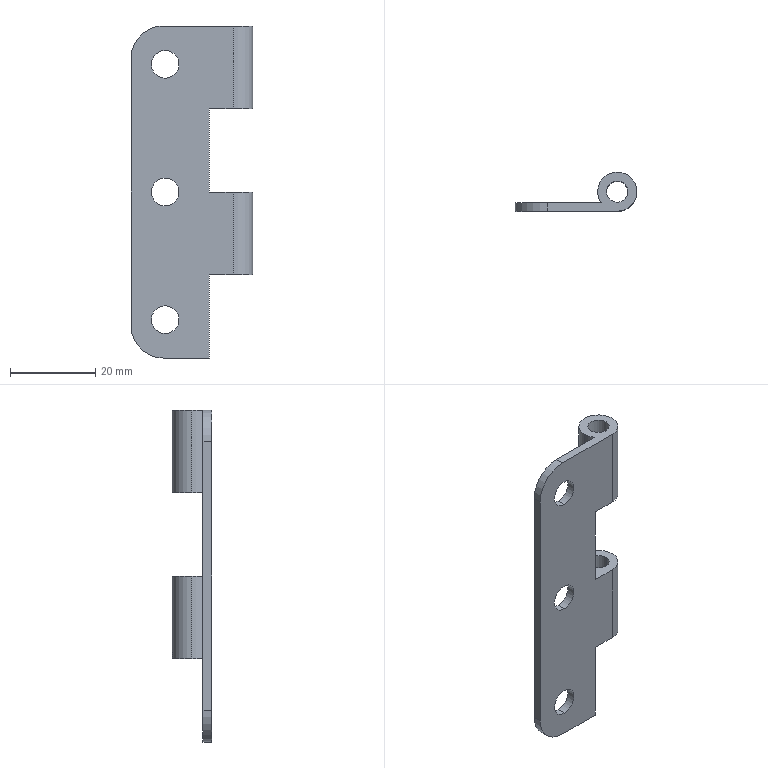Part | SolidWorks | features BaseBody 1 | 1 solid | 28 faces | box 28.6 x 9.2 x 78 mm | volume 4679 mm3 | cylinder 18 | plane 10 | commonest cylinder face diameters 6.5 x6 9.2 x6 5 x4 15 x2
STEP:
#1=CARTESIAN_POINT('',(-16.,2.,-33.25));
#2=VERTEX_POINT('',#1);
#3=CARTESIAN_POINT('',(-16.,2.,-26.75));
#4=VERTEX_POINT('',#3);
#5=CARTESIAN_POINT('',(-16.,2.,-30.));
#6=DIRECTION('',(0.,1.,0.));
#7=DIRECTION('',(0.,0.,1.));
#8=AXIS2_PLACEMENT_3D('',#5,#6,#7);
#9=CIRCLE('',#8,3.25);
#10=EDGE_CURVE('',#2,#4,#9,.T.);
#11=ORIENTED_EDGE('',*,*,#10,.T.);
#12=CARTESIAN_POINT('',(-16.,0.,-26.75));
#13=VERTEX_POINT('',#12);
#14=CARTESIAN_POINT('',(-16.,2.,-26.75));
#15=DIRECTION('',(0.,-1.,0.));
#16=VECTOR('',#15,1000.);
#17=LINE('',#14,#16);
#18=EDGE_CURVE('',#4,#13,#17,.T.);
#19=ORIENTED_EDGE('',*,*,#18,.T.);
#20=CARTESIAN_POINT('',(-16.,0.,-33.25));
#21=VERTEX_POINT('',#20);
#22=CARTESIAN_POINT('',(-16.,0.,-30.));
#23=DIRECTION('',(0.,1.,0.));
#24=DIRECTION('',(0.,0.,1.));
#25=AXIS2_PLACEMENT_3D('',#22,#23,#24);
#26=CIRCLE('',#25,3.25);
#27=EDGE_CURVE('',#21,#13,#26,.T.);
#28=ORIENTED_EDGE('',*,*,#27,.F.);
#29=CARTESIAN_POINT('',(-16.,2.,-33.25));
#30=DIRECTION('',(0.,-1.,0.));
#31=VECTOR('',#30,1000.);
#32=LINE('',#29,#31);
#33=EDGE_CURVE('',#2,#21,#32,.T.);
#34=ORIENTED_EDGE('',*,*,#33,.F.);
#35=EDGE_LOOP('',(#11,#19,#28,#34));
#36=FACE_OUTER_BOUND('',#35,.T.);
#37=CARTESIAN_POINT('',(-16.,2.,-30.));
#38=DIRECTION('',(0.,-1.,0.));
#39=DIRECTION('',(0.,0.,-1.));
#40=AXIS2_PLACEMENT_3D('',#37,#38,#39);
#41=CYLINDRICAL_SURFACE('',#40,3.25);
#42=ADVANCED_FACE('',(#36),#41,.F.);
#43=CARTESIAN_POINT('',(-16.,2.,26.75));
#44=VERTEX_POINT('',#43);
#45=CARTESIAN_POINT('',(-16.,2.,33.25));
#46=VERTEX_POINT('',#45);
#47=CARTESIAN_POINT('',(-16.,2.,30.));
#48=DIRECTION('',(0.,1.,0.));
#49=DIRECTION('',(0.,0.,1.));
#50=AXIS2_PLACEMENT_3D('',#47,#48,#49);
#51=CIRCLE('',#50,3.25);
#52=EDGE_CURVE('',#44,#46,#51,.T.);
#53=ORIENTED_EDGE('',*,*,#52,.T.);
#54=CARTESIAN_POINT('',(-16.,0.,33.25));
#55=VERTEX_POINT('',#54);
#56=CARTESIAN_POINT('',(-16.,2.,33.25));
#57=DIRECTION('',(0.,-1.,0.));
#58=VECTOR('',#57,1000.);
#59=LINE('',#56,#58);
#60=EDGE_CURVE('',#46,#55,#59,.T.);
#61=ORIENTED_EDGE('',*,*,#60,.T.);
#62=CARTESIAN_POINT('',(-16.,0.,26.75));
#63=VERTEX_POINT('',#62);
#64=CARTESIAN_POINT('',(-16.,0.,30.));
#65=DIRECTION('',(0.,1.,0.));
#66=DIRECTION('',(0.,0.,1.));
#67=AXIS2_PLACEMENT_3D('',#64,#65,#66);
#68=CIRCLE('',#67,3.25);
#69=EDGE_CURVE('',#63,#55,#68,.T.);
#70=ORIENTED_EDGE('',*,*,#69,.F.);
#71=CARTESIAN_POINT('',(-16.,2.,26.75));
#72=DIRECTION('',(0.,-1.,0.));
#73=VECTOR('',#72,1000.);
#74=LINE('',#71,#73);
#75=EDGE_CURVE('',#44,#63,#74,.T.);
#76=ORIENTED_EDGE('',*,*,#75,.F.);
#77=EDGE_LOOP('',(#53,#61,#70,#76));
#78=FACE_OUTER_BOUND('',#77,.T.);
#79=CARTESIAN_POINT('',(-16.,2.,30.));
#80=DIRECTION('',(0.,-1.,0.));
#81=DIRECTION('',(0.,0.,-1.));
#82=AXIS2_PLACEMENT_3D('',#79,#80,#81);
#83=CYLINDRICAL_SURFACE('',#82,3.25);
#84=ADVANCED_FACE('',(#78),#83,.F.);
#85=CARTESIAN_POINT('',(-16.,2.,-3.25));
#86=VERTEX_POINT('',#85);
#87=CARTESIAN_POINT('',(-16.,2.,3.25));
#88=VERTEX_POINT('',#87);
#89=CARTESIAN_POINT('',(-16.,2.,0.));
#90=DIRECTION('',(0.,1.,0.));
#91=DIRECTION('',(0.,0.,1.));
#92=AXIS2_PLACEMENT_3D('',#89,#90,#91);
#93=CIRCLE('',#92,3.25);
#94=EDGE_CURVE('',#86,#88,#93,.T.);
#95=ORIENTED_EDGE('',*,*,#94,.T.);
#96=CARTESIAN_POINT('',(-16.,0.,3.25));
#97=VERTEX_POINT('',#96);
#98=CARTESIAN_POINT('',(-16.,2.,3.25));
#99=DIRECTION('',(0.,-1.,0.));
#100=VECTOR('',#99,1000.);
#101=LINE('',#98,#100);
#102=EDGE_CURVE('',#88,#97,#101,.T.);
#103=ORIENTED_EDGE('',*,*,#102,.T.);
#104=CARTESIAN_POINT('',(-16.,0.,-3.25));
#105=VERTEX_POINT('',#104);
#106=CARTESIAN_POINT('',(-16.,0.,0.));
#107=DIRECTION('',(0.,1.,0.));
#108=DIRECTION('',(0.,0.,1.));
#109=AXIS2_PLACEMENT_3D('',#106,#107,#108);
#110=CIRCLE('',#109,3.25);
#111=EDGE_CURVE('',#105,#97,#110,.T.);
#112=ORIENTED_EDGE('',*,*,#111,.F.);
#113=CARTESIAN_POINT('',(-16.,2.,-3.25));
#114=DIRECTION('',(0.,-1.,0.));
#115=VECTOR('',#114,1000.);
#116=LINE('',#113,#115);
#117=EDGE_CURVE('',#86,#105,#116,.T.);
#118=ORIENTED_EDGE('',*,*,#117,.F.);
#119=EDGE_LOOP('',(#95,#103,#112,#118));
#120=FACE_OUTER_BOUND('',#119,.T.);
#121=CARTESIAN_POINT('',(-16.,2.,0.));
#122=DIRECTION('',(0.,-1.,0.));
#123=DIRECTION('',(0.,0.,-1.));
#124=AXIS2_PLACEMENT_3D('',#121,#122,#123);
#125=CYLINDRICAL_SURFACE('',#124,3.25);
#126=ADVANCED_FACE('',(#120),#125,.F.);
#127=CARTESIAN_POINT('',(-2.5,4.6,-19.5));
#128=VERTEX_POINT('',#127);
#129=CARTESIAN_POINT('',(2.5,4.6,-19.5));
#130=VERTEX_POINT('',#129);
#131=CARTESIAN_POINT('',(0.,4.6,-19.5));
#132=DIRECTION('',(0.,0.,1.));
#133=DIRECTION('',(-1.,0.,0.));
#134=AXIS2_PLACEMENT_3D('',#131,#132,#133);
#135=CIRCLE('',#134,2.5);
#136=EDGE_CURVE('',#128,#130,#135,.T.);
#137=ORIENTED_EDGE('',*,*,#136,.F.);
#138=CARTESIAN_POINT('',(-2.5,4.6,0.));
#139=VERTEX_POINT('',#138);
#140=CARTESIAN_POINT('',(-2.5,4.6,-39.));
#141=DIRECTION('',(0.,0.,1.));
#142=VECTOR('',#141,1000.);
#143=LINE('',#140,#142);
#144=EDGE_CURVE('',#128,#139,#143,.T.);
#145=ORIENTED_EDGE('',*,*,#144,.T.);
#146=CARTESIAN_POINT('',(2.5,4.6,0.));
#147=VERTEX_POINT('',#146);
#148=CARTESIAN_POINT('',(0.,4.6,0.));
#149=DIRECTION('',(0.,0.,-1.));
#150=DIRECTION('',(1.,0.,0.));
#151=AXIS2_PLACEMENT_3D('',#148,#149,#150);
#152=CIRCLE('',#151,2.5);
#153=EDGE_CURVE('',#147,#139,#152,.T.);
#154=ORIENTED_EDGE('',*,*,#153,.F.);
#155=CARTESIAN_POINT('',(2.5,4.6,-39.));
#156=DIRECTION('',(0.,0.,1.));
#157=VECTOR('',#156,1000.);
#158=LINE('',#155,#157);
#159=EDGE_CURVE('',#130,#147,#158,.T.);
#160=ORIENTED_EDGE('',*,*,#159,.F.);
#161=EDGE_LOOP('',(#137,#145,#154,#160));
#162=FACE_OUTER_BOUND('',#161,.T.);
#163=CARTESIAN_POINT('',(0.,4.6,-39.));
#164=DIRECTION('',(0.,0.,1.));
#165=DIRECTION('',(1.,0.,0.));
#166=AXIS2_PLACEMENT_3D('',#163,#164,#165);
#167=CYLINDRICAL_SURFACE('',#166,2.5);
#168=ADVANCED_FACE('',(#162),#167,.F.);
#169=CARTESIAN_POINT('',(-2.5,4.6,19.5));
#170=VERTEX_POINT('',#169);
#171=CARTESIAN_POINT('',(2.5,4.6,19.5));
#172=VERTEX_POINT('',#171);
#173=CARTESIAN_POINT('',(0.,4.6,19.5));
#174=DIRECTION('',(0.,0.,1.));
#175=DIRECTION('',(-1.,0.,0.));
#176=AXIS2_PLACEMENT_3D('',#173,#174,#175);
#177=CIRCLE('',#176,2.5);
#178=EDGE_CURVE('',#170,#172,#177,.T.);
#179=ORIENTED_EDGE('',*,*,#178,.F.);
#180=CARTESIAN_POINT('',(-2.5,4.6,39.));
#181=VERTEX_POINT('',#180);
#182=CARTESIAN_POINT('',(-2.5,4.6,-39.));
#183=DIRECTION('',(0.,0.,1.));
#184=VECTOR('',#183,1000.);
#185=LINE('',#182,#184);
#186=EDGE_CURVE('',#170,#181,#185,.T.);
#187=ORIENTED_EDGE('',*,*,#186,.T.);
#188=CARTESIAN_POINT('',(2.5,4.6,39.));
#189=VERTEX_POINT('',#188);
#190=CARTESIAN_POINT('',(0.,4.6,39.));
#191=DIRECTION('',(0.,0.,1.));
#192=DIRECTION('',(1.,0.,0.));
#193=AXIS2_PLACEMENT_3D('',#190,#191,#192);
#194=CIRCLE('',#193,2.5);
#195=EDGE_CURVE('',#181,#189,#194,.T.);
#196=ORIENTED_EDGE('',*,*,#195,.T.);
#197=CARTESIAN_POINT('',(2.5,4.6,-39.));
#198=DIRECTION('',(0.,0.,1.));
#199=VECTOR('',#198,1000.);
#200=LINE('',#197,#199);
#201=EDGE_CURVE('',#172,#189,#200,.T.);
#202=ORIENTED_EDGE('',*,*,#201,.F.);
#203=EDGE_LOOP('',(#179,#187,#196,#202));
#204=FACE_OUTER_BOUND('',#203,.T.);
#205=CARTESIAN_POINT('',(0.,4.6,-39.));
#206=DIRECTION('',(0.,0.,1.));
#207=DIRECTION('',(1.,0.,0.));
#208=AXIS2_PLACEMENT_3D('',#205,#206,#207);
#209=CYLINDRICAL_SURFACE('',#208,2.5);
#210=ADVANCED_FACE('',(#204),#209,.F.);
#211=CARTESIAN_POINT('',(4.6,4.6,-19.5));
#212=VERTEX_POINT('',#211);
#213=CARTESIAN_POINT('',(-4.6,4.6,-19.5));
#214=VERTEX_POINT('',#213);
#215=CARTESIAN_POINT('',(0.,4.6,-19.5));
#216=DIRECTION('',(0.,0.,1.));
#217=DIRECTION('',(-1.,0.,0.));
#218=AXIS2_PLACEMENT_3D('',#215,#216,#217);
#219=CIRCLE('',#218,4.6);
#220=EDGE_CURVE('',#212,#214,#219,.T.);
#221=ORIENTED_EDGE('',*,*,#220,.T.);
#222=CARTESIAN_POINT('',(-4.6,4.6,0.));
#223=VERTEX_POINT('',#222);
#224=CARTESIAN_POINT('',(-4.6,4.6,-39.));
#225=DIRECTION('',(0.,0.,1.));
#226=VECTOR('',#225,1000.);
#227=LINE('',#224,#226);
#228=EDGE_CURVE('',#214,#223,#227,.T.);
#229=ORIENTED_EDGE('',*,*,#228,.T.);
#230=CARTESIAN_POINT('',(4.6,4.6,0.));
#231=VERTEX_POINT('',#230);
#232=CARTESIAN_POINT('',(0.,4.6,0.));
#233=DIRECTION('',(0.,0.,-1.));
#234=DIRECTION('',(1.,0.,0.));
#235=AXIS2_PLACEMENT_3D('',#232,#233,#234);
#236=CIRCLE('',#235,4.6);
#237=EDGE_CURVE('',#223,#231,#236,.T.);
#238=ORIENTED_EDGE('',*,*,#237,.T.);
#239=CARTESIAN_POINT('',(4.6,4.6,-39.));
#240=DIRECTION('',(0.,0.,1.));
#241=VECTOR('',#240,1000.);
#242=LINE('',#239,#241);
#243=EDGE_CURVE('',#212,#231,#242,.T.);
#244=ORIENTED_EDGE('',*,*,#243,.F.);
#245=EDGE_LOOP('',(#221,#229,#238,#244));
#246=FACE_OUTER_BOUND('',#245,.T.);
#247=CARTESIAN_POINT('',(0.,4.6,-39.));
#248=DIRECTION('',(0.,0.,1.));
#249=DIRECTION('',(1.,0.,0.));
#250=AXIS2_PLACEMENT_3D('',#247,#248,#249);
#251=CYLINDRICAL_SURFACE('',#250,4.6);
#252=ADVANCED_FACE('',(#246),#251,.T.);
#253=CARTESIAN_POINT('',(0.,0.,-19.5));
#254=VERTEX_POINT('',#253);
#255=CARTESIAN_POINT('',(0.,4.6,-19.5));
#256=DIRECTION('',(0.,0.,1.));
#257=DIRECTION('',(-1.,0.,0.));
#258=AXIS2_PLACEMENT_3D('',#255,#256,#257);
#259=CIRCLE('',#258,4.6);
#260=EDGE_CURVE('',#254,#212,#259,.T.);
#261=ORIENTED_EDGE('',*,*,#260,.T.);
#262=ORIENTED_EDGE('',*,*,#243,.T.);
#263=CARTESIAN_POINT('',(0.,0.,0.));
#264=VERTEX_POINT('',#263);
#265=CARTESIAN_POINT('',(0.,4.6,0.));
#266=DIRECTION('',(0.,0.,-1.));
#267=DIRECTION('',(1.,0.,0.));
#268=AXIS2_PLACEMENT_3D('',#265,#266,#267);
#269=CIRCLE('',#268,4.6);
#270=EDGE_CURVE('',#231,#264,#269,.T.);
#271=ORIENTED_EDGE('',*,*,#270,.T.);
#272=CARTESIAN_POINT('',(0.,0.,-39.));
#273=DIRECTION('',(0.,0.,-1.));
#274=VECTOR('',#273,1000.);
#275=LINE('',#272,#274);
#276=EDGE_CURVE('',#264,#254,#275,.T.);
#277=ORIENTED_EDGE('',*,*,#276,.T.);
#278=EDGE_LOOP('',(#261,#262,#271,#277));
#279=FACE_OUTER_BOUND('',#278,.T.);
#280=CARTESIAN_POINT('',(0.,4.6,-39.));
#281=DIRECTION('',(0.,0.,1.));
#282=DIRECTION('',(1.,0.,0.));
#283=AXIS2_PLACEMENT_3D('',#280,#281,#282);
#284=CYLINDRICAL_SURFACE('',#283,4.6);
#285=ADVANCED_FACE('',(#279),#284,.T.);
#286=CARTESIAN_POINT('',(4.6,4.6,19.5));
#287=VERTEX_POINT('',#286);
#288=CARTESIAN_POINT('',(-4.6,4.6,19.5));
#289=VERTEX_POINT('',#288);
#290=CARTESIAN_POINT('',(0.,4.6,19.5));
#291=DIRECTION('',(0.,0.,1.));
#292=DIRECTION('',(-1.,0.,0.));
#293=AXIS2_PLACEMENT_3D('',#290,#291,#292);
#294=CIRCLE('',#293,4.6);
#295=EDGE_CURVE('',#287,#289,#294,.T.);
#296=ORIENTED_EDGE('',*,*,#295,.T.);
#297=CARTESIAN_POINT('',(-4.6,4.6,39.));
#298=VERTEX_POINT('',#297);
#299=CARTESIAN_POINT('',(-4.6,4.6,-39.));
#300=DIRECTION('',(0.,0.,1.));
#301=VECTOR('',#300,1000.);
#302=LINE('',#299,#301);
#303=EDGE_CURVE('',#289,#298,#302,.T.);
#304=ORIENTED_EDGE('',*,*,#303,.T.);
#305=CARTESIAN_POINT('',(4.6,4.6,39.));
#306=VERTEX_POINT('',#305);
#307=CARTESIAN_POINT('',(0.,4.6,39.));
#308=DIRECTION('',(0.,0.,1.));
#309=DIRECTION('',(1.,0.,0.));
#310=AXIS2_PLACEMENT_3D('',#307,#308,#309);
#311=CIRCLE('',#310,4.6);
#312=EDGE_CURVE('',#306,#298,#311,.T.);
#313=ORIENTED_EDGE('',*,*,#312,.F.);
#314=CARTESIAN_POINT('',(4.6,4.6,-39.));
#315=DIRECTION('',(0.,0.,1.));
#316=VECTOR('',#315,1000.);
#317=LINE('',#314,#316);
#318=EDGE_CURVE('',#287,#306,#317,.T.);
#319=ORIENTED_EDGE('',*,*,#318,.F.);
#320=EDGE_LOOP('',(#296,#304,#313,#319));
#321=FACE_OUTER_BOUND('',#320,.T.);
#322=CARTESIAN_POINT('',(0.,4.6,-39.));
#323=DIRECTION('',(0.,0.,1.));
#324=DIRECTION('',(1.,0.,0.));
#325=AXIS2_PLACEMENT_3D('',#322,#323,#324);
#326=CYLINDRICAL_SURFACE('',#325,4.6);
#327=ADVANCED_FACE('',(#321),#326,.T.);
#328=CARTESIAN_POINT('',(0.,0.,19.5));
#329=VERTEX_POINT('',#328);
#330=CARTESIAN_POINT('',(0.,4.6,19.5));
#331=DIRECTION('',(0.,0.,1.));
#332=DIRECTION('',(-1.,0.,0.));
#333=AXIS2_PLACEMENT_3D('',#330,#331,#332);
#334=CIRCLE('',#333,4.6);
#335=EDGE_CURVE('',#329,#287,#334,.T.);
#336=ORIENTED_EDGE('',*,*,#335,.T.);
#337=ORIENTED_EDGE('',*,*,#318,.T.);
#338=CARTESIAN_POINT('',(0.,0.,39.));
#339=VERTEX_POINT('',#338);
#340=CARTESIAN_POINT('',(0.,4.6,39.));
#341=DIRECTION('',(0.,0.,1.));
#342=DIRECTION('',(1.,0.,0.));
#343=AXIS2_PLACEMENT_3D('',#340,#341,#342);
#344=CIRCLE('',#343,4.6);
#345=EDGE_CURVE('',#339,#306,#344,.T.);
#346=ORIENTED_EDGE('',*,*,#345,.F.);
#347=CARTESIAN_POINT('',(0.,0.,-39.));
#348=DIRECTION('',(0.,0.,-1.));
#349=VECTOR('',#348,1000.);
#350=LINE('',#347,#349);
#351=EDGE_CURVE('',#339,#329,#350,.T.);
#352=ORIENTED_EDGE('',*,*,#351,.T.);
#353=EDGE_LOOP('',(#336,#337,#346,#352));
#354=FACE_OUTER_BOUND('',#353,.T.);
#355=CARTESIAN_POINT('',(0.,4.6,-39.));
#356=DIRECTION('',(0.,0.,1.));
#357=DIRECTION('',(1.,0.,0.));
#358=AXIS2_PLACEMENT_3D('',#355,#356,#357);
#359=CYLINDRICAL_SURFACE('',#358,4.6);
#360=ADVANCED_FACE('',(#354),#359,.T.);
#361=CARTESIAN_POINT('',(-3.795,2.,19.5));
#362=VERTEX_POINT('',#361);
#363=CARTESIAN_POINT('',(-3.795,2.,39.));
#364=VERTEX_POINT('',#363);
#365=CARTESIAN_POINT('',(-3.795,2.,-39.));
#366=DIRECTION('',(0.,0.,1.));
#367=VECTOR('',#366,1000.);
#368=LINE('',#365,#367);
#369=EDGE_CURVE('',#362,#364,#368,.T.);
#370=ORIENTED_EDGE('',*,*,#369,.F.);
#371=CARTESIAN_POINT('',(-5.6,2.,19.5));
#372=VERTEX_POINT('',#371);
#373=CARTESIAN_POINT('',(-16.5,2.,19.5));
#374=DIRECTION('',(-1.,0.,0.));
#375=VECTOR('',#374,1000.);
#376=LINE('',#373,#375);
#377=EDGE_CURVE('',#362,#372,#376,.T.);
#378=ORIENTED_EDGE('',*,*,#377,.T.);
#379=CARTESIAN_POINT('',(-5.6,2.,0.));
#380=VERTEX_POINT('',#379);
#381=CARTESIAN_POINT('',(-5.6,2.,31.5));
#382=DIRECTION('',(0.,0.,-1.));
#383=VECTOR('',#382,1000.);
#384=LINE('',#381,#383);
#385=EDGE_CURVE('',#372,#380,#384,.T.);
#386=ORIENTED_EDGE('',*,*,#385,.T.);
#387=CARTESIAN_POINT('',(-3.795,2.,0.));
#388=VERTEX_POINT('',#387);
#389=CARTESIAN_POINT('',(-16.5,2.,0.));
#390=DIRECTION('',(1.,0.,0.));
#391=VECTOR('',#390,1000.);
#392=LINE('',#389,#391);
#393=EDGE_CURVE('',#380,#388,#392,.T.);
#394=ORIENTED_EDGE('',*,*,#393,.T.);
#395=CARTESIAN_POINT('',(-3.795,2.,-19.5));
#396=VERTEX_POINT('',#395);
#397=CARTESIAN_POINT('',(-3.795,2.,-39.));
#398=DIRECTION('',(0.,0.,1.));
#399=VECTOR('',#398,1000.);
#400=LINE('',#397,#399);
#401=EDGE_CURVE('',#396,#388,#400,.T.);
#402=ORIENTED_EDGE('',*,*,#401,.F.);
#403=CARTESIAN_POINT('',(-5.6,2.,-19.5));
#404=VERTEX_POINT('',#403);
#405=CARTESIAN_POINT('',(-16.5,2.,-19.5));
#406=DIRECTION('',(-1.,0.,0.));
#407=VECTOR('',#406,1000.);
#408=LINE('',#405,#407);
#409=EDGE_CURVE('',#396,#404,#408,.T.);
#410=ORIENTED_EDGE('',*,*,#409,.T.);
#411=CARTESIAN_POINT('',(-5.6,2.,-39.));
#412=VERTEX_POINT('',#411);
#413=CARTESIAN_POINT('',(-5.6,2.,31.5));
#414=DIRECTION('',(0.,0.,-1.));
#415=VECTOR('',#414,1000.);
#416=LINE('',#413,#415);
#417=EDGE_CURVE('',#404,#412,#416,.T.);
#418=ORIENTED_EDGE('',*,*,#417,.T.);
#419=CARTESIAN_POINT('',(-16.5,2.,-39.));
#420=VERTEX_POINT('',#419);
#421=CARTESIAN_POINT('',(-16.5,2.,-39.));
#422=DIRECTION('',(-1.,0.,0.));
#423=VECTOR('',#422,1000.);
#424=LINE('',#421,#423);
#425=EDGE_CURVE('',#412,#420,#424,.T.);
#426=ORIENTED_EDGE('',*,*,#425,.T.);
#427=CARTESIAN_POINT('',(-24.,2.,-31.5));
#428=VERTEX_POINT('',#427);
#429=CARTESIAN_POINT('',(-16.5,2.,-31.5));
#430=DIRECTION('',(0.,1.,0.));
#431=DIRECTION('',(0.,0.,1.));
#432=AXIS2_PLACEMENT_3D('',#429,#430,#431);
#433=CIRCLE('',#432,7.5);
#434=EDGE_CURVE('',#420,#428,#433,.T.);
#435=ORIENTED_EDGE('',*,*,#434,.T.);
#436=CARTESIAN_POINT('',(-24.,2.,31.5));
#437=VERTEX_POINT('',#436);
#438=CARTESIAN_POINT('',(-24.,2.,-31.5));
#439=DIRECTION('',(0.,0.,1.));
#440=VECTOR('',#439,1000.);
#441=LINE('',#438,#440);
#442=EDGE_CURVE('',#428,#437,#441,.T.);
#443=ORIENTED_EDGE('',*,*,#442,.T.);
#444=CARTESIAN_POINT('',(-16.5,2.,39.));
#445=VERTEX_POINT('',#444);
#446=CARTESIAN_POINT('',(-16.5,2.,31.5));
#447=DIRECTION('',(0.,1.,0.));
#448=DIRECTION('',(0.,0.,1.));
#449=AXIS2_PLACEMENT_3D('',#446,#447,#448);
#450=CIRCLE('',#449,7.5);
#451=EDGE_CURVE('',#437,#445,#450,.T.);
#452=ORIENTED_EDGE('',*,*,#451,.T.);
#453=CARTESIAN_POINT('',(-16.5,2.,39.));
#454=DIRECTION('',(1.,0.,0.));
#455=VECTOR('',#454,1000.);
#456=LINE('',#453,#455);
#457=EDGE_CURVE('',#445,#364,#456,.T.);
#458=ORIENTED_EDGE('',*,*,#457,.T.);
#459=EDGE_LOOP('',(#370,#378,#386,#394,#402,#410,#418,#426,#435,#443,#452,#458));
#460=FACE_OUTER_BOUND('',#459,.T.);
#461=ORIENTED_EDGE('',*,*,#52,.F.);
#462=CARTESIAN_POINT('',(-16.,2.,30.));
#463=DIRECTION('',(0.,1.,0.));
#464=DIRECTION('',(0.,0.,1.));
#465=AXIS2_PLACEMENT_3D('',#462,#463,#464);
#466=CIRCLE('',#465,3.25);
#467=EDGE_CURVE('',#46,#44,#466,.T.);
#468=ORIENTED_EDGE('',*,*,#467,.F.);
#469=EDGE_LOOP('',(#461,#468));
#470=FACE_BOUND('',#469,.T.);
#471=ORIENTED_EDGE('',*,*,#94,.F.);
#472=CARTESIAN_POINT('',(-16.,2.,0.));
#473=DIRECTION('',(0.,1.,0.));
#474=DIRECTION('',(0.,0.,1.));
#475=AXIS2_PLACEMENT_3D('',#472,#473,#474);
#476=CIRCLE('',#475,3.25);
#477=EDGE_CURVE('',#88,#86,#476,.T.);
#478=ORIENTED_EDGE('',*,*,#477,.F.);
#479=EDGE_LOOP('',(#471,#478));
#480=FACE_BOUND('',#479,.T.);
#481=ORIENTED_EDGE('',*,*,#10,.F.);
#482=CARTESIAN_POINT('',(-16.,2.,-30.));
#483=DIRECTION('',(0.,1.,0.));
#484=DIRECTION('',(0.,0.,1.));
#485=AXIS2_PLACEMENT_3D('',#482,#483,#484);
#486=CIRCLE('',#485,3.25);
#487=EDGE_CURVE('',#4,#2,#486,.T.);
#488=ORIENTED_EDGE('',*,*,#487,.F.);
#489=EDGE_LOOP('',(#481,#488));
#490=FACE_BOUND('',#489,.T.);
#491=CARTESIAN_POINT('',(-16.5,2.,31.5));
#492=DIRECTION('',(0.,1.,0.));
#493=DIRECTION('',(0.,0.,1.));
#494=AXIS2_PLACEMENT_3D('',#491,#492,#493);
#495=PLANE('',#494);
#496=ADVANCED_FACE('',(#460,#470,#480,#490),#495,.T.);
#497=ORIENTED_EDGE('',*,*,#111,.T.);
#498=CARTESIAN_POINT('',(-16.,0.,0.));
#499=DIRECTION('',(0.,1.,0.));
#500=DIRECTION('',(0.,0.,1.));
#501=AXIS2_PLACEMENT_3D('',#498,#499,#500);
#502=CIRCLE('',#501,3.25);
#503=EDGE_CURVE('',#97,#105,#502,.T.);
#504=ORIENTED_EDGE('',*,*,#503,.T.);
#505=EDGE_LOOP('',(#497,#504));
#506=FACE_BOUND('',#505,.T.);
#507=ORIENTED_EDGE('',*,*,#69,.T.);
#508=CARTESIAN_POINT('',(-16.,0.,30.));
#509=DIRECTION('',(0.,1.,0.));
#510=DIRECTION('',(0.,0.,1.));
#511=AXIS2_PLACEMENT_3D('',#508,#509,#510);
#512=CIRCLE('',#511,3.25);
#513=EDGE_CURVE('',#55,#63,#512,.T.);
#514=ORIENTED_EDGE('',*,*,#513,.T.);
#515=EDGE_LOOP('',(#507,#514));
#516=FACE_BOUND('',#515,.T.);
#517=CARTESIAN_POINT('',(-5.6,0.,19.5));
#518=VERTEX_POINT('',#517);
#519=CARTESIAN_POINT('',(-5.6,0.,19.5));
#520=DIRECTION('',(1.,0.,0.));
#521=VECTOR('',#520,1000.);
#522=LINE('',#519,#521);
#523=EDGE_CURVE('',#518,#329,#522,.T.);
#524=ORIENTED_EDGE('',*,*,#523,.T.);
#525=ORIENTED_EDGE('',*,*,#351,.F.);
#526=CARTESIAN_POINT('',(-16.5,0.,39.));
#527=VERTEX_POINT('',#526);
#528=CARTESIAN_POINT('',(-16.5,0.,39.));
#529=DIRECTION('',(1.,0.,0.));
#530=VECTOR('',#529,1000.);
#531=LINE('',#528,#530);
#532=EDGE_CURVE('',#527,#339,#531,.T.);
#533=ORIENTED_EDGE('',*,*,#532,.F.);
#534=CARTESIAN_POINT('',(-24.,0.,31.5));
#535=VERTEX_POINT('',#534);
#536=CARTESIAN_POINT('',(-16.5,0.,31.5));
#537=DIRECTION('',(0.,1.,0.));
#538=DIRECTION('',(0.,0.,1.));
#539=AXIS2_PLACEMENT_3D('',#536,#537,#538);
#540=CIRCLE('',#539,7.5);
#541=EDGE_CURVE('',#535,#527,#540,.T.);
#542=ORIENTED_EDGE('',*,*,#541,.F.);
#543=CARTESIAN_POINT('',(-24.,0.,-31.5));
#544=VERTEX_POINT('',#543);
#545=CARTESIAN_POINT('',(-24.,0.,-31.5));
#546=DIRECTION('',(0.,0.,1.));
#547=VECTOR('',#546,1000.);
#548=LINE('',#545,#547);
#549=EDGE_CURVE('',#544,#535,#548,.T.);
#550=ORIENTED_EDGE('',*,*,#549,.F.);
#551=CARTESIAN_POINT('',(-16.5,0.,-39.));
#552=VERTEX_POINT('',#551);
#553=CARTESIAN_POINT('',(-16.5,0.,-31.5));
#554=DIRECTION('',(0.,1.,0.));
#555=DIRECTION('',(0.,0.,1.));
#556=AXIS2_PLACEMENT_3D('',#553,#554,#555);
#557=CIRCLE('',#556,7.5);
#558=EDGE_CURVE('',#552,#544,#557,.T.);
#559=ORIENTED_EDGE('',*,*,#558,.F.);
#560=CARTESIAN_POINT('',(-5.6,0.,-39.));
#561=VERTEX_POINT('',#560);
#562=CARTESIAN_POINT('',(-16.5,0.,-39.));
#563=DIRECTION('',(-1.,0.,0.));
#564=VECTOR('',#563,1000.);
#565=LINE('',#562,#564);
#566=EDGE_CURVE('',#561,#552,#565,.T.);
#567=ORIENTED_EDGE('',*,*,#566,.F.);
#568=CARTESIAN_POINT('',(-5.6,0.,-19.5));
#569=VERTEX_POINT('',#568);
#570=CARTESIAN_POINT('',(-5.6,0.,-19.5));
#571=DIRECTION('',(0.,0.,1.));
#572=VECTOR('',#571,1000.);
#573=LINE('',#570,#572);
#574=EDGE_CURVE('',#561,#569,#573,.T.);
#575=ORIENTED_EDGE('',*,*,#574,.T.);
#576=CARTESIAN_POINT('',(-5.6,0.,-19.5));
#577=DIRECTION('',(1.,0.,0.));
#578=VECTOR('',#577,1000.);
#579=LINE('',#576,#578);
#580=EDGE_CURVE('',#569,#254,#579,.T.);
#581=ORIENTED_EDGE('',*,*,#580,.T.);
#582=ORIENTED_EDGE('',*,*,#276,.F.);
#583=CARTESIAN_POINT('',(-5.6,0.,0.));
#584=VERTEX_POINT('',#583);
#585=CARTESIAN_POINT('',(-5.6,0.,0.));
#586=DIRECTION('',(-1.,0.,0.));
#587=VECTOR('',#586,1000.);
#588=LINE('',#585,#587);
#589=EDGE_CURVE('',#264,#584,#588,.T.);
#590=ORIENTED_EDGE('',*,*,#589,.T.);
#591=CARTESIAN_POINT('',(-5.6,0.,19.5));
#592=DIRECTION('',(0.,0.,1.));
#593=VECTOR('',#592,1000.);
#594=LINE('',#591,#593);
#595=EDGE_CURVE('',#584,#518,#594,.T.);
#596=ORIENTED_EDGE('',*,*,#595,.T.);
#597=EDGE_LOOP('',(#524,#525,#533,#542,#550,#559,#567,#575,#581,#582,#590,#596));
#598=FACE_OUTER_BOUND('',#597,.T.);
#599=ORIENTED_EDGE('',*,*,#27,.T.);
#600=CARTESIAN_POINT('',(-16.,0.,-30.));
#601=DIRECTION('',(0.,1.,0.));
#602=DIRECTION('',(0.,0.,1.));
#603=AXIS2_PLACEMENT_3D('',#600,#601,#602);
#604=CIRCLE('',#603,3.25);
#605=EDGE_CURVE('',#13,#21,#604,.T.);
#606=ORIENTED_EDGE('',*,*,#605,.T.);
#607=EDGE_LOOP('',(#599,#606));
#608=FACE_BOUND('',#607,.T.);
#609=CARTESIAN_POINT('',(-16.5,0.,31.5));
#610=DIRECTION('',(0.,1.,0.));
#611=DIRECTION('',(0.,0.,1.));
#612=AXIS2_PLACEMENT_3D('',#609,#610,#611);
#613=PLANE('',#612);
#614=ADVANCED_FACE('',(#506,#516,#598,#608),#613,.F.);
#615=ORIENTED_EDGE('',*,*,#303,.F.);
#616=CARTESIAN_POINT('',(0.,4.6,19.5));
#617=DIRECTION('',(0.,0.,1.));
#618=DIRECTION('',(-1.,0.,0.));
#619=AXIS2_PLACEMENT_3D('',#616,#617,#618);
#620=CIRCLE('',#619,4.6);
#621=EDGE_CURVE('',#289,#362,#620,.T.);
#622=ORIENTED_EDGE('',*,*,#621,.T.);
#623=ORIENTED_EDGE('',*,*,#369,.T.);
#624=CARTESIAN_POINT('',(0.,4.6,39.));
#625=DIRECTION('',(0.,0.,1.));
#626=DIRECTION('',(1.,0.,0.));
#627=AXIS2_PLACEMENT_3D('',#624,#625,#626);
#628=CIRCLE('',#627,4.6);
#629=EDGE_CURVE('',#298,#364,#628,.T.);
#630=ORIENTED_EDGE('',*,*,#629,.F.);
#631=EDGE_LOOP('',(#615,#622,#623,#630));
#632=FACE_OUTER_BOUND('',#631,.T.);
#633=CARTESIAN_POINT('',(0.,4.6,-39.));
#634=DIRECTION('',(0.,0.,1.));
#635=DIRECTION('',(1.,0.,0.));
#636=AXIS2_PLACEMENT_3D('',#633,#634,#635);
#637=CYLINDRICAL_SURFACE('',#636,4.6);
#638=ADVANCED_FACE('',(#632),#637,.T.);
#639=ORIENTED_EDGE('',*,*,#228,.F.);
#640=CARTESIAN_POINT('',(0.,4.6,-19.5));
#641=DIRECTION('',(0.,0.,1.));
#642=DIRECTION('',(-1.,0.,0.));
#643=AXIS2_PLACEMENT_3D('',#640,#641,#642);
#644=CIRCLE('',#643,4.6);
#645=EDGE_CURVE('',#214,#396,#644,.T.);
#646=ORIENTED_EDGE('',*,*,#645,.T.);
#647=ORIENTED_EDGE('',*,*,#401,.T.);
#648=CARTESIAN_POINT('',(0.,4.6,0.));
#649=DIRECTION('',(0.,0.,-1.));
#650=DIRECTION('',(1.,0.,0.));
#651=AXIS2_PLACEMENT_3D('',#648,#649,#650);
#652=CIRCLE('',#651,4.6);
#653=EDGE_CURVE('',#388,#223,#652,.T.);
#654=ORIENTED_EDGE('',*,*,#653,.T.);
#655=EDGE_LOOP('',(#639,#646,#647,#654));
#656=FACE_OUTER_BOUND('',#655,.T.);
#657=CARTESIAN_POINT('',(0.,4.6,-39.));
#658=DIRECTION('',(0.,0.,1.));
#659=DIRECTION('',(1.,0.,0.));
#660=AXIS2_PLACEMENT_3D('',#657,#658,#659);
#661=CYLINDRICAL_SURFACE('',#660,4.6);
#662=ADVANCED_FACE('',(#656),#661,.T.);
#663=ORIENTED_EDGE('',*,*,#186,.F.);
#664=CARTESIAN_POINT('',(0.,4.6,19.5));
#665=DIRECTION('',(0.,0.,1.));
#666=DIRECTION('',(-1.,0.,0.));
#667=AXIS2_PLACEMENT_3D('',#664,#665,#666);
#668=CIRCLE('',#667,2.5);
#669=EDGE_CURVE('',#172,#170,#668,.T.);
#670=ORIENTED_EDGE('',*,*,#669,.F.);
#671=ORIENTED_EDGE('',*,*,#201,.T.);
#672=CARTESIAN_POINT('',(0.,4.6,39.));
#673=DIRECTION('',(0.,0.,1.));
#674=DIRECTION('',(1.,0.,0.));
#675=AXIS2_PLACEMENT_3D('',#672,#673,#674);
#676=CIRCLE('',#675,2.5);
#677=EDGE_CURVE('',#189,#181,#676,.T.);
#678=ORIENTED_EDGE('',*,*,#677,.T.);
#679=EDGE_LOOP('',(#663,#670,#671,#678));
#680=FACE_OUTER_BOUND('',#679,.T.);
#681=CARTESIAN_POINT('',(0.,4.6,-39.));
#682=DIRECTION('',(0.,0.,1.));
#683=DIRECTION('',(1.,0.,0.));
#684=AXIS2_PLACEMENT_3D('',#681,#682,#683);
#685=CYLINDRICAL_SURFACE('',#684,2.5);
#686=ADVANCED_FACE('',(#680),#685,.F.);
#687=ORIENTED_EDGE('',*,*,#144,.F.);
#688=CARTESIAN_POINT('',(0.,4.6,-19.5));
#689=DIRECTION('',(0.,0.,1.));
#690=DIRECTION('',(-1.,0.,0.));
#691=AXIS2_PLACEMENT_3D('',#688,#689,#690);
#692=CIRCLE('',#691,2.5);
#693=EDGE_CURVE('',#130,#128,#692,.T.);
#694=ORIENTED_EDGE('',*,*,#693,.F.);
#695=ORIENTED_EDGE('',*,*,#159,.T.);
#696=CARTESIAN_POINT('',(0.,4.6,0.));
#697=DIRECTION('',(0.,0.,-1.));
#698=DIRECTION('',(1.,0.,0.));
#699=AXIS2_PLACEMENT_3D('',#696,#697,#698);
#700=CIRCLE('',#699,2.5);
#701=EDGE_CURVE('',#139,#147,#700,.T.);
#702=ORIENTED_EDGE('',*,*,#701,.F.);
#703=EDGE_LOOP('',(#687,#694,#695,#702));
#704=FACE_OUTER_BOUND('',#703,.T.);
#705=CARTESIAN_POINT('',(0.,4.6,-39.));
#706=DIRECTION('',(0.,0.,1.));
#707=DIRECTION('',(1.,0.,0.));
#708=AXIS2_PLACEMENT_3D('',#705,#706,#707);
#709=CYLINDRICAL_SURFACE('',#708,2.5);
#710=ADVANCED_FACE('',(#704),#709,.F.);
#711=CARTESIAN_POINT('',(-5.6,9.2,-39.));
#712=DIRECTION('',(0.,-1.,0.));
#713=VECTOR('',#712,1000.);
#714=LINE('',#711,#713);
#715=EDGE_CURVE('',#412,#561,#714,.T.);
#716=ORIENTED_EDGE('',*,*,#715,.T.);
#717=ORIENTED_EDGE('',*,*,#566,.T.);
#718=CARTESIAN_POINT('',(-16.5,2.,-39.));
#719=DIRECTION('',(0.,-1.,0.));
#720=VECTOR('',#719,1000.);
#721=LINE('',#718,#720);
#722=EDGE_CURVE('',#420,#552,#721,.T.);
#723=ORIENTED_EDGE('',*,*,#722,.F.);
#724=ORIENTED_EDGE('',*,*,#425,.F.);
#725=EDGE_LOOP('',(#716,#717,#723,#724));
#726=FACE_OUTER_BOUND('',#725,.T.);
#727=CARTESIAN_POINT('',(-16.5,2.,-39.));
#728=DIRECTION('',(0.,0.,1.));
#729=DIRECTION('',(1.,0.,0.));
#730=AXIS2_PLACEMENT_3D('',#727,#728,#729);
#731=PLANE('',#730);
#732=ADVANCED_FACE('',(#726),#731,.F.);
#733=ORIENTED_EDGE('',*,*,#541,.T.);
#734=CARTESIAN_POINT('',(-16.5,2.,39.));
#735=DIRECTION('',(0.,-1.,0.));
#736=VECTOR('',#735,1000.);
#737=LINE('',#734,#736);
#738=EDGE_CURVE('',#445,#527,#737,.T.);
#739=ORIENTED_EDGE('',*,*,#738,.F.);
#740=ORIENTED_EDGE('',*,*,#451,.F.);
#741=CARTESIAN_POINT('',(-24.,2.,31.5));
#742=DIRECTION('',(0.,-1.,0.));
#743=VECTOR('',#742,1000.);
#744=LINE('',#741,#743);
#745=EDGE_CURVE('',#437,#535,#744,.T.);
#746=ORIENTED_EDGE('',*,*,#745,.T.);
#747=EDGE_LOOP('',(#733,#739,#740,#746));
#748=FACE_OUTER_BOUND('',#747,.T.);
#749=CARTESIAN_POINT('',(-16.5,2.,31.5));
#750=DIRECTION('',(0.,-1.,0.));
#751=DIRECTION('',(0.,0.,-1.));
#752=AXIS2_PLACEMENT_3D('',#749,#750,#751);
#753=CYLINDRICAL_SURFACE('',#752,7.5);
#754=ADVANCED_FACE('',(#748),#753,.T.);
#755=ORIENTED_EDGE('',*,*,#677,.F.);
#756=ORIENTED_EDGE('',*,*,#195,.F.);
#757=EDGE_LOOP('',(#755,#756));
#758=FACE_BOUND('',#757,.T.);
#759=ORIENTED_EDGE('',*,*,#532,.T.);
#760=ORIENTED_EDGE('',*,*,#345,.T.);
#761=ORIENTED_EDGE('',*,*,#312,.T.);
#762=ORIENTED_EDGE('',*,*,#629,.T.);
#763=ORIENTED_EDGE('',*,*,#457,.F.);
#764=ORIENTED_EDGE('',*,*,#738,.T.);
#765=EDGE_LOOP('',(#759,#760,#761,#762,#763,#764));
#766=FACE_OUTER_BOUND('',#765,.T.);
#767=CARTESIAN_POINT('',(-16.5,2.,39.));
#768=DIRECTION('',(0.,0.,-1.));
#769=DIRECTION('',(-1.,0.,0.));
#770=AXIS2_PLACEMENT_3D('',#767,#768,#769);
#771=PLANE('',#770);
#772=ADVANCED_FACE('',(#758,#766),#771,.F.);
#773=ORIENTED_EDGE('',*,*,#558,.T.);
#774=CARTESIAN_POINT('',(-24.,2.,-31.5));
#775=DIRECTION('',(0.,-1.,0.));
#776=VECTOR('',#775,1000.);
#777=LINE('',#774,#776);
#778=EDGE_CURVE('',#428,#544,#777,.T.);
#779=ORIENTED_EDGE('',*,*,#778,.F.);
#780=ORIENTED_EDGE('',*,*,#434,.F.);
#781=ORIENTED_EDGE('',*,*,#722,.T.);
#782=EDGE_LOOP('',(#773,#779,#780,#781));
#783=FACE_OUTER_BOUND('',#782,.T.);
#784=CARTESIAN_POINT('',(-16.5,2.,-31.5));
#785=DIRECTION('',(0.,-1.,0.));
#786=DIRECTION('',(0.,0.,-1.));
#787=AXIS2_PLACEMENT_3D('',#784,#785,#786);
#788=CYLINDRICAL_SURFACE('',#787,7.5);
#789=ADVANCED_FACE('',(#783),#788,.T.);
#790=ORIENTED_EDGE('',*,*,#549,.T.);
#791=ORIENTED_EDGE('',*,*,#745,.F.);
#792=ORIENTED_EDGE('',*,*,#442,.F.);
#793=ORIENTED_EDGE('',*,*,#778,.T.);
#794=EDGE_LOOP('',(#790,#791,#792,#793));
#795=FACE_OUTER_BOUND('',#794,.T.);
#796=CARTESIAN_POINT('',(-24.,2.,-31.5));
#797=DIRECTION('',(1.,0.,0.));
#798=DIRECTION('',(0.,0.,-1.));
#799=AXIS2_PLACEMENT_3D('',#796,#797,#798);
#800=PLANE('',#799);
#801=ADVANCED_FACE('',(#795),#800,.F.);
#802=ORIENTED_EDGE('',*,*,#102,.F.);
#803=ORIENTED_EDGE('',*,*,#477,.T.);
#804=ORIENTED_EDGE('',*,*,#117,.T.);
#805=ORIENTED_EDGE('',*,*,#503,.F.);
#806=EDGE_LOOP('',(#802,#803,#804,#805));
#807=FACE_OUTER_BOUND('',#806,.T.);
#808=CARTESIAN_POINT('',(-16.,2.,0.));
#809=DIRECTION('',(0.,-1.,0.));
#810=DIRECTION('',(0.,0.,-1.));
#811=AXIS2_PLACEMENT_3D('',#808,#809,#810);
#812=CYLINDRICAL_SURFACE('',#811,3.25);
#813=ADVANCED_FACE('',(#807),#812,.F.);
#814=ORIENTED_EDGE('',*,*,#60,.F.);
#815=ORIENTED_EDGE('',*,*,#467,.T.);
#816=ORIENTED_EDGE('',*,*,#75,.T.);
#817=ORIENTED_EDGE('',*,*,#513,.F.);
#818=EDGE_LOOP('',(#814,#815,#816,#817));
#819=FACE_OUTER_BOUND('',#818,.T.);
#820=CARTESIAN_POINT('',(-16.,2.,30.));
#821=DIRECTION('',(0.,-1.,0.));
#822=DIRECTION('',(0.,0.,-1.));
#823=AXIS2_PLACEMENT_3D('',#820,#821,#822);
#824=CYLINDRICAL_SURFACE('',#823,3.25);
#825=ADVANCED_FACE('',(#819),#824,.F.);
#826=ORIENTED_EDGE('',*,*,#260,.F.);
#827=ORIENTED_EDGE('',*,*,#580,.F.);
#828=CARTESIAN_POINT('',(-5.6,9.2,-19.5));
#829=DIRECTION('',(0.,-1.,0.));
#830=VECTOR('',#829,1000.);
#831=LINE('',#828,#830);
#832=EDGE_CURVE('',#404,#569,#831,.T.);
#833=ORIENTED_EDGE('',*,*,#832,.F.);
#834=ORIENTED_EDGE('',*,*,#409,.F.);
#835=ORIENTED_EDGE('',*,*,#645,.F.);
#836=ORIENTED_EDGE('',*,*,#220,.F.);
#837=EDGE_LOOP('',(#826,#827,#833,#834,#835,#836));
#838=FACE_OUTER_BOUND('',#837,.T.);
#839=ORIENTED_EDGE('',*,*,#693,.T.);
#840=ORIENTED_EDGE('',*,*,#136,.T.);
#841=EDGE_LOOP('',(#839,#840));
#842=FACE_BOUND('',#841,.T.);
#843=CARTESIAN_POINT('',(-5.6,9.2,-19.5));
#844=DIRECTION('',(0.,0.,-1.));
#845=DIRECTION('',(-1.,0.,0.));
#846=AXIS2_PLACEMENT_3D('',#843,#844,#845);
#847=PLANE('',#846);
#848=ADVANCED_FACE('',(#838,#842),#847,.T.);
#849=ORIENTED_EDGE('',*,*,#832,.T.);
#850=ORIENTED_EDGE('',*,*,#574,.F.);
#851=ORIENTED_EDGE('',*,*,#715,.F.);
#852=ORIENTED_EDGE('',*,*,#417,.F.);
#853=EDGE_LOOP('',(#849,#850,#851,#852));
#854=FACE_OUTER_BOUND('',#853,.T.);
#855=CARTESIAN_POINT('',(-5.6,9.2,-19.5));
#856=DIRECTION('',(1.,0.,0.));
#857=DIRECTION('',(0.,0.,-1.));
#858=AXIS2_PLACEMENT_3D('',#855,#856,#857);
#859=PLANE('',#858);
#860=ADVANCED_FACE('',(#854),#859,.T.);
#861=ORIENTED_EDGE('',*,*,#335,.F.);
#862=ORIENTED_EDGE('',*,*,#523,.F.);
#863=CARTESIAN_POINT('',(-5.6,9.2,19.5));
#864=DIRECTION('',(0.,-1.,0.));
#865=VECTOR('',#864,1000.);
#866=LINE('',#863,#865);
#867=EDGE_CURVE('',#372,#518,#866,.T.);
#868=ORIENTED_EDGE('',*,*,#867,.F.);
#869=ORIENTED_EDGE('',*,*,#377,.F.);
#870=ORIENTED_EDGE('',*,*,#621,.F.);
#871=ORIENTED_EDGE('',*,*,#295,.F.);
#872=EDGE_LOOP('',(#861,#862,#868,#869,#870,#871));
#873=FACE_OUTER_BOUND('',#872,.T.);
#874=ORIENTED_EDGE('',*,*,#669,.T.);
#875=ORIENTED_EDGE('',*,*,#178,.T.);
#876=EDGE_LOOP('',(#874,#875));
#877=FACE_BOUND('',#876,.T.);
#878=CARTESIAN_POINT('',(-5.6,9.2,19.5));
#879=DIRECTION('',(0.,0.,-1.));
#880=DIRECTION('',(-1.,0.,0.));
#881=AXIS2_PLACEMENT_3D('',#878,#879,#880);
#882=PLANE('',#881);
#883=ADVANCED_FACE('',(#873,#877),#882,.T.);
#884=CARTESIAN_POINT('',(-5.6,9.2,0.));
#885=DIRECTION('',(0.,-1.,0.));
#886=VECTOR('',#885,1000.);
#887=LINE('',#884,#886);
#888=EDGE_CURVE('',#380,#584,#887,.T.);
#889=ORIENTED_EDGE('',*,*,#888,.T.);
#890=ORIENTED_EDGE('',*,*,#589,.F.);
#891=ORIENTED_EDGE('',*,*,#270,.F.);
#892=ORIENTED_EDGE('',*,*,#237,.F.);
#893=ORIENTED_EDGE('',*,*,#653,.F.);
#894=ORIENTED_EDGE('',*,*,#393,.F.);
#895=EDGE_LOOP('',(#889,#890,#891,#892,#893,#894));
#896=FACE_OUTER_BOUND('',#895,.T.);
#897=ORIENTED_EDGE('',*,*,#153,.T.);
#898=ORIENTED_EDGE('',*,*,#701,.T.);
#899=EDGE_LOOP('',(#897,#898));
#900=FACE_BOUND('',#899,.T.);
#901=CARTESIAN_POINT('',(-5.6,9.2,0.));
#902=DIRECTION('',(0.,0.,1.));
#903=DIRECTION('',(1.,0.,0.));
#904=AXIS2_PLACEMENT_3D('',#901,#902,#903);
#905=PLANE('',#904);
#906=ADVANCED_FACE('',(#896,#900),#905,.T.);
#907=ORIENTED_EDGE('',*,*,#867,.T.);
#908=ORIENTED_EDGE('',*,*,#595,.F.);
#909=ORIENTED_EDGE('',*,*,#888,.F.);
#910=ORIENTED_EDGE('',*,*,#385,.F.);
#911=EDGE_LOOP('',(#907,#908,#909,#910));
#912=FACE_OUTER_BOUND('',#911,.T.);
#913=CARTESIAN_POINT('',(-5.6,9.2,19.5));
#914=DIRECTION('',(1.,0.,0.));
#915=DIRECTION('',(0.,0.,-1.));
#916=AXIS2_PLACEMENT_3D('',#913,#914,#915);
#917=PLANE('',#916);
#918=ADVANCED_FACE('',(#912),#917,.T.);
#919=ORIENTED_EDGE('',*,*,#18,.F.);
#920=ORIENTED_EDGE('',*,*,#487,.T.);
#921=ORIENTED_EDGE('',*,*,#33,.T.);
#922=ORIENTED_EDGE('',*,*,#605,.F.);
#923=EDGE_LOOP('',(#919,#920,#921,#922));
#924=FACE_OUTER_BOUND('',#923,.T.);
#925=CARTESIAN_POINT('',(-16.,2.,-30.));
#926=DIRECTION('',(0.,-1.,0.));
#927=DIRECTION('',(0.,0.,-1.));
#928=AXIS2_PLACEMENT_3D('',#925,#926,#927);
#929=CYLINDRICAL_SURFACE('',#928,3.25);
#930=ADVANCED_FACE('',(#924),#929,.F.);
#931=CLOSED_SHELL('',(#42,#84,#126,#168,#210,#252,#285,#327,#360,#496,#614,#638,#662,#686,#710,#732,#754,#772,#789,#801,#813,#825,#848,#860,#883,#906,#918,#930));
#932=MANIFOLD_SOLID_BREP('',#931);
#933=CARTESIAN_POINT('',(0.,0.,0.));
#934=DIRECTION('',(0.,0.,1.));
#935=DIRECTION('',(1.,0.,0.));
#936=AXIS2_PLACEMENT_3D('',#933,#934,#935);
#937=(LENGTH_UNIT()NAMED_UNIT(*)SI_UNIT(.MILLI.,.METRE.));
#938=UNCERTAINTY_MEASURE_WITH_UNIT(LENGTH_MEASURE(0.00001),#937,'','');
#939=(NAMED_UNIT(*)PLANE_ANGLE_UNIT()SI_UNIT($,.RADIAN.));
#940=(NAMED_UNIT(*)SI_UNIT($,.STERADIAN.)SOLID_ANGLE_UNIT());
#941=(GEOMETRIC_REPRESENTATION_CONTEXT(3)GLOBAL_UNCERTAINTY_ASSIGNED_CONTEXT((#938))GLOBAL_UNIT_ASSIGNED_CONTEXT((#937,#939,#940))REPRESENTATION_CONTEXT('',''));
#942=ADVANCED_BREP_SHAPE_REPRESENTATION('',(#932,#936),#941);